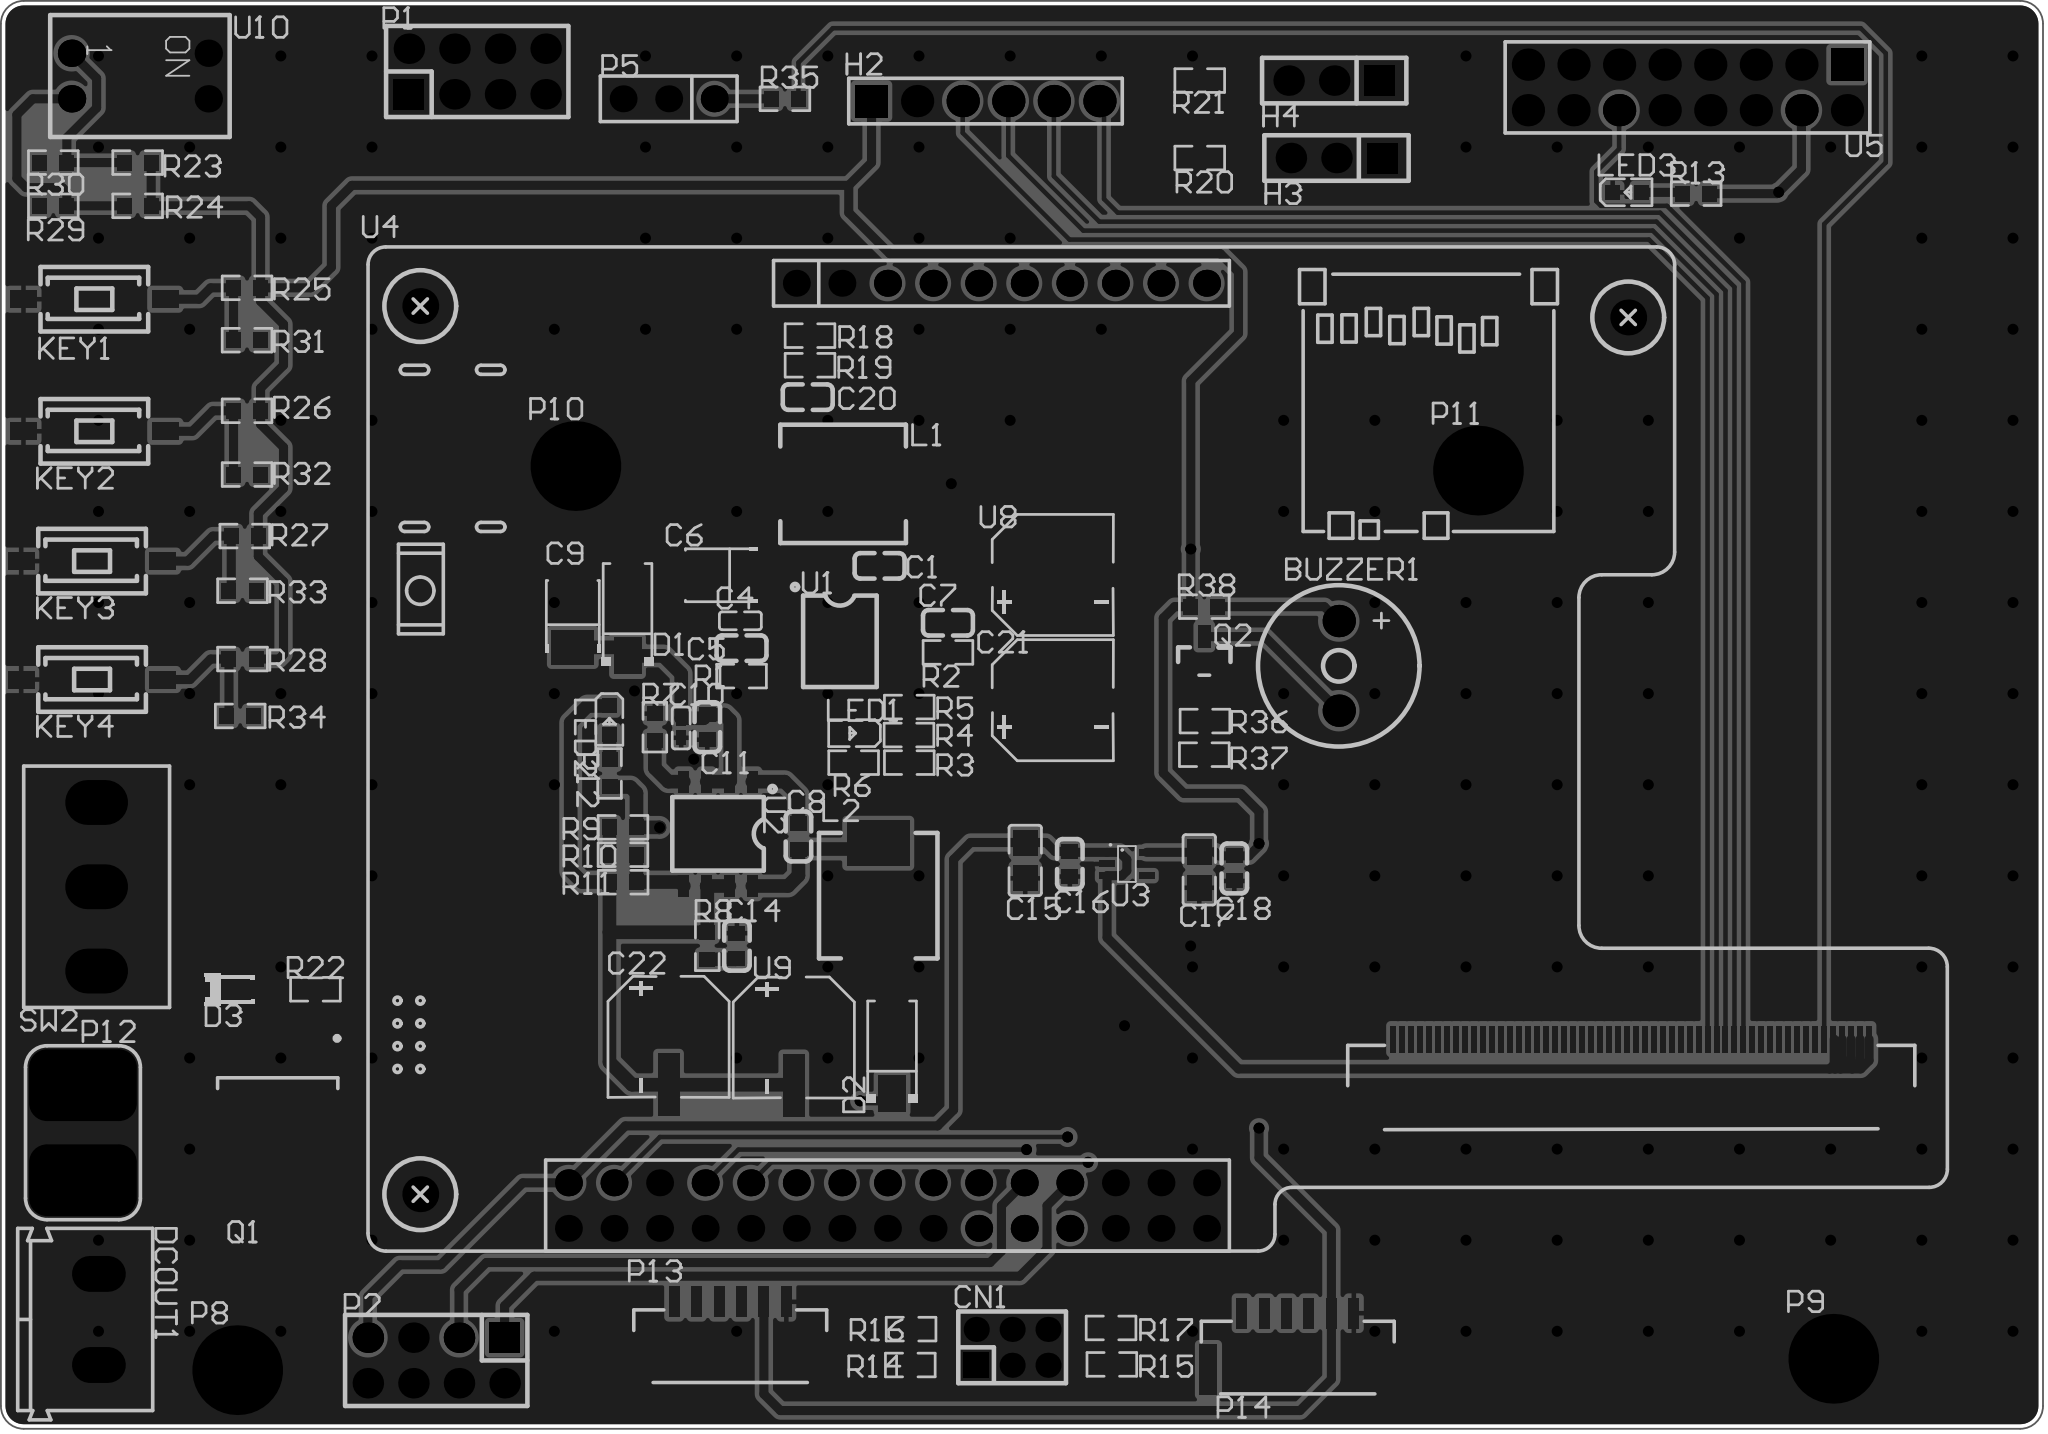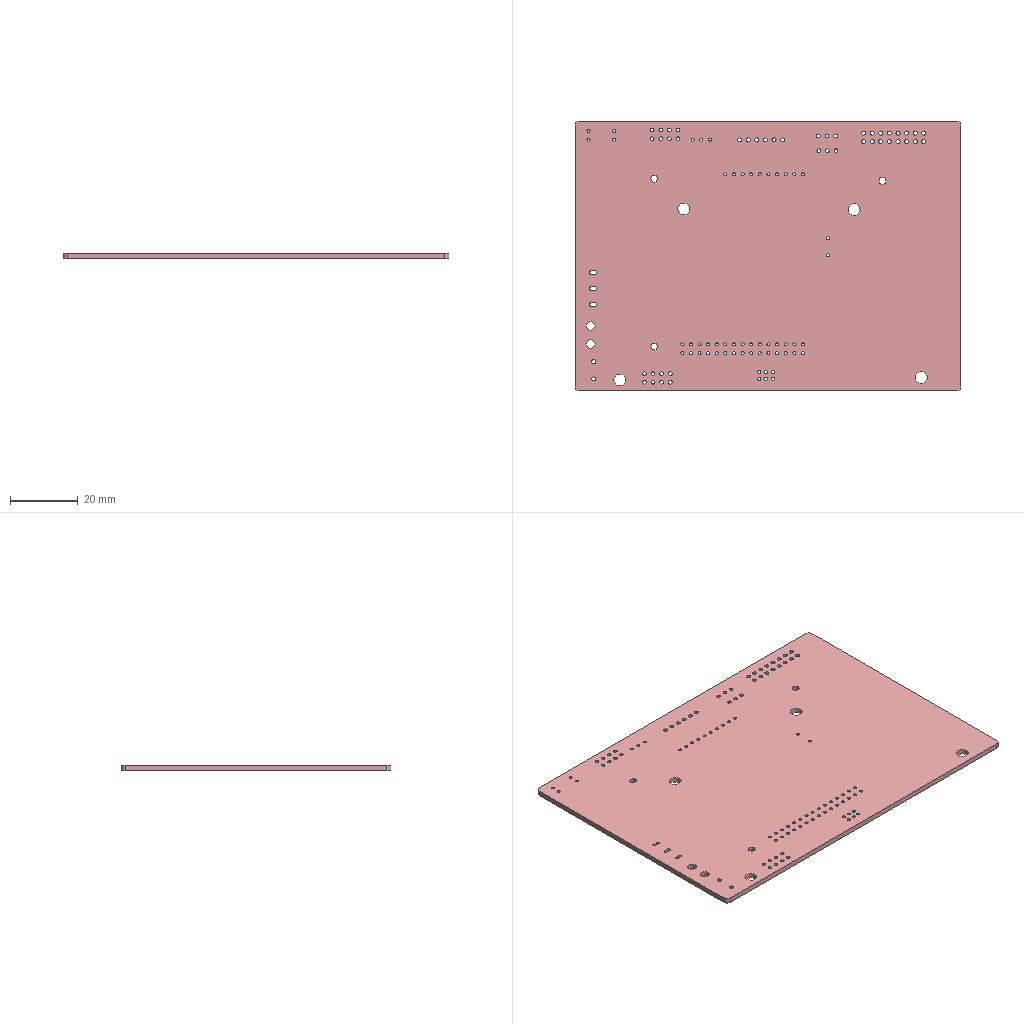Circuit board layout | Altium Designer | box 113.8 x 79.6 x 1.6 mm
Layer stack:
# Altium Designer layer stack of  (unit mm; dielectric type: 0 none, 1 core, 2 prepreg, 3 surface material)
index,name,kind,layer,copper_thickness_mm,dielectric_type,dielectric_thickness_mm,dielectric_material,dielectric_constant
0,Top Paste Mask Layer,other,,,,,,
1,Top Silkscreen Layer,other,,,,,,
2,Top Solder Mask Layer,dielectric,,,3,0.01,,3.3
3,Top Layer,copper,Top Layer,0.035,,,,
4,Dielectric1,dielectric,,,3,1.51,FR4,4.5
5,Bottom Layer,copper,Bottom Layer,0.035,,,,
6,Bottom Solder Mask Layer,dielectric,,,3,0.01,,3.3
7,Bottom Silkscreen Layer,other,,,,,,
8,Bottom Paste Mask Layer,other,,,,,,
# drill layer pairs: low layer,high layer
drill_pair,Top Layer,Bottom Layer
Part placement:
Designator,Comment,Layer,Footprint,Center-X(mm),Center-Y(mm),Rotation
BUZZER1,BEEP,TopLayer,BUZ-TH_BD9-P50-D0.6-FD,159.512,130.683,270
C1,100nF,TopLayer,C0603,133.925,136.26,0
C4,4.7uF,TopLayer,C0402,126.167,133.196,0
C5,100nF,TopLayer,C0603,126.232,131.672,0
C6,100uF,TopLayer,CAP-SMD_L3.5-W2.8-R-RD,124.934,135.736,0
C7,4.7nF,TopLayer,C0603,137.735,133.085,0
C8,100nF,TopLayer,C0603,129.405,121.169,270
C9,100uF,TopLayer,CAP-SMD_L3.5-W2.8-R-RD,116.832,133.615,270
C10,4.7uF,TopLayer,C0402,122.871,127.218,90
C11,100nF,TopLayer,C0603,124.325,127.265,90
C14,4.7nF,TopLayer,C0603,125.975,115.076,270
C15,10uF,TopLayer,C0805,142.04,119.833,90
C16,100nF,TopLayer,C0603,144.526,119.634,90
C17,10uF,TopLayer,C0805,151.738,119.309,90
C18,100nF,TopLayer,C0603,153.692,119.387,90
CN1,A2005WV-2x3P,TopLayer,HDR-TH_6P-P2.00-V-M-R2-C3-S2.00,141.311,92.679,0
D1,SS54,TopLayer,SMA_L4.4-W2.8-LS5.4-R-RD,119.879,133.742,90
D2,SS54,TopLayer,SMA_L4.4-W2.8-LS5.4-R-RD,134.62,109.347,90
D3,BZT52C16,TopLayer,SOD-123-L,97.79,112.649,180
DCOUT1,DCOUT1,TopLayer,KF/WJ/DG_301-2P-5.0MM,90.424,94.234,90
H2,2.54-1x6P straight pin,TopLayer,HDR-TH_6P-P2.54-V-M-1,139.827,162.179,0
H3,,TopLayer,HDR-TH_3P-P2.54-V-M,159.385,159.004,180
H4,,TopLayer,HDR-TH_3P-P2.54-V-M,159.258,163.322,180
KEY1,Tact switch 3x6x2.5mm,TopLayer,SW-SMD_L6.0-W3.6-LS8.0,90.17,151.13,180
KEY2,Tact switch 3x6x2.5mm,TopLayer,SW-SMD_L6.0-W3.6-LS8.0,90.17,143.764,180
KEY3,Tact switch 3x6x2.5mm,TopLayer,SW-SMD_L6.0-W3.6-LS8.0,90.043,136.525,180
KEY4,Tact switch 3x6x2.5mm,TopLayer,SW-SMD_L6.0-W3.6-LS8.0,90.043,129.921,180
LED1,LTST-C190KSKT,TopLayer,LED0603-RD,132.478,126.937,180
LED2,LTST-C190KSKT,TopLayer,LED0603-RD,118.864,127.646,270
LED3,LTST-C190KSKT,TopLayer,LED0603-RD,175.574,157.088,0
P1,Straight header 2X4P 2.54mm,TopLayer,HDR-TH_8P-P2.54-V-M-R2-C4-S2.54,111.506,163.83,0
P2,Straight header 2X4P 2.54mm,TopLayer,HDR-TH_8P-P2.54-V-M-R2-C4-S2.54,109.22,91.948,180
P5,Header-D-M 1x3P,TopLayer,HDR1X3-M,122.174,162.306,180
P8,,TopLayer,定位孔,98.13,91.406,0
P9,,TopLayer,定位孔,187.069,92.041,0
P10,,TopLayer,定位孔,116.976,141.825,0
P11,,TopLayer,定位孔,167.268,141.571,0
P12,XT60_Header,TopLayer,Wired_T-Header_ThroughHole,89.535,104.648,0
P13,GH1.25-6P,TopLayer,ECD-GH1.25-6P-SH,125.603,93.643,0
P14,GH1.25-6P,TopLayer,ECD-GH1.25-6P-SH,157.226,93.008,0
Q1,HY19P03,TopLayer,TO-252AA,100.387,106.635,270
Q2,S8050,TopLayer,SOT-23(SOT-23-3),152.019,131.064,0
SW2,SS-12D10L9,TopLayer,MTS-10x,90.297,118.364,90
U1,SCT2450CQSTER,TopLayer,ESOP-8_L4.9-W3.9-P1.27-LS6.0-BL-EP,131.713,132.053,270
U2,SCT2450CQSTER,TopLayer,ESOP-8_L4.9-W3.9-P1.27-LS6.0-BL-EP,124.924,121.316,180
U3,RT9013-33GU5,TopLayer,SC-70-5_L2.0-W1.3-P0.65-LS2.1-BR,147.701,119.634,180
U4,Loongson 2K0300 development board,TopLayer,龙芯2K0300久久派开发板,149.746,125.666,0
U5,2X8PIN2.54,TopLayer,HDR-TH_16P-P2.54-V-M-R2-C8-S2.54,178.943,162.941,180
R1,200kΩ,TopLayer,R0603,126.232,130.112,0
R2,20kΩ,TopLayer,R0603,137.735,131.434,0
R3,27kΩ,TopLayer,R0603,135.58,125.288,180
R4,27kΩ,TopLayer,R0603,135.563,126.826,0
R5,7.5kΩ,TopLayer,R0603,135.58,128.386,180
R6,10K,TopLayer,R0603,132.478,125.286,0
R7,200kΩ,TopLayer,R0603,121.403,127.265,270
R8,20kΩ,TopLayer,R0603,124.325,115.073,270
R9,51kΩ,TopLayer,R0603,119.626,121.677,0
R10,1.5kΩ,TopLayer,R0603,119.626,120.153,180
R11,7.5kΩ,TopLayer,R0603,119.634,118.618,0
R12,4.7kΩ,TopLayer,R0603,118.876,124.682,270
R13,2.7kΩ,TopLayer,R0603,179.427,157.017,180
R14,100Ω,TopLayer,R0603,135.636,91.694,0
R15,100Ω,TopLayer,R0603,146.867,91.728,180
R16,100Ω,TopLayer,R0603,135.679,93.695,180
R17,100Ω,TopLayer,R0603,146.823,93.76,0
R18,20kΩ,TopLayer,R0603,130.048,149.098,0
R19,200kΩ,TopLayer,R0603,130.048,147.447,180
R20,100Ω,TopLayer,R0603,151.765,159.004,180
R21,100Ω,TopLayer,R0603,151.765,163.322,180
R22,10K,TopLayer,R0603,102.489,112.649,180
R23,4.7kΩ,TopLayer,R0603,92.583,158.75,180
R24,4.7kΩ,TopLayer,R0603,92.583,156.337,180
R25,4.7kΩ,TopLayer,R0603,98.679,151.765,180
R26,4.7kΩ,TopLayer,R0603,98.679,144.907,180
R27,4.7kΩ,TopLayer,R0603,98.552,137.922,180
R28,4.7kΩ,TopLayer,R0603,98.425,131.064,180
R29,470Ω,TopLayer,R0603,87.884,156.337,180
R30,470Ω,TopLayer,R0603,87.884,158.75,180
R31,100Ω,TopLayer,R0603,98.679,148.844,0
R32,100Ω,TopLayer,R0603,98.679,141.351,0
R33,100Ω,TopLayer,R0603,98.425,134.874,0
R34,100Ω,TopLayer,R0603,98.298,127.889,0
R35,100Ω,TopLayer,R0603,128.651,162.306,180
R36,4.7kΩ,TopLayer,R0603,152.056,127.604,180
R37,1kΩ,TopLayer,R0603,152.019,125.73,180
R38,10Ω,TopLayer,R0603,152.019,133.985,0
C20,100nF,TopLayer,C0603,129.921,145.669,0
C21,47uF,TopLayer,CAP-SMD_BD6.3-L6.6-W6.6-LS7.3-FD,143.577,128.767,0
C22,47uF,TopLayer,CAP-SMD_BD6.3-L6.6-W6.6-LS7.3-FD,122.165,109.993,270
U8,220uF,TopLayer,CAP-SMD_BD6.3-L6.6-W6.6-LS7.2-FD,143.577,135.752,0
U9,220uF,TopLayer,CAP-SMD_BD6.3-L6.6-W6.6-LS7.2-FD,129.144,109.955,270
L1,4.7uH,TopLayer,IND-SMD_L7.0-W6.6_VCMT063T,131.893,140.832,0
L2,4.7uH,TopLayer,IND-SMD_L7.0-W6.6_VCMT063T,133.85,117.867,270
U10,2-position DIP switch,TopLayer,SW-TH_4P-L9.9-W6.8-P7.62-BL,92.71,163.576,270
Pad and via stacks:
# Altium Designer via and pad stacks of  (unit mm). Each distinct definition once, with the count of objects using it.
# via: kind,start_layer,end_layer,hole_mm,diameter_mm,mode(0 simple;1 top-mid-bottom;2 full stack),diameter_per_layer,count,example_net
# pad: kind,layer,hole_mm,hole_type(0 round;1 square;2 slot),plating,top_size,top_shape(1 round;2 rect;3 octagon;9 rounded rect),mid_size,bottom_size,mode,footprint,size_per_layer,count,example
pad,Multi-Layer,1,0,plated,1.8x1.8,1,1.8x1.8,1.8x1.8,0,BUZ-TH_BD9-P50-D0.6-FD,,2,BUZZER1.2
pad,Multi-Layer,0.9,0,plated,1.4x1.4,1,1.4x1.4,1.4x1.4,0,HDR-TH_6P-P2.00-V-M-R2-C3-S2.00,,5,CN1.6
pad,Multi-Layer,0.9,0,plated,1.4x1.4,2,1.4x1.4,1.4x1.4,0,HDR-TH_6P-P2.00-V-M-R2-C3-S2.00,,1,CN1.1
pad,Multi-Layer,1.2,0,plated,2x3,1,2x3,2x3,0,KF/WJ/DG 301-2P-5.0MM,,2,DCOUT1.1
pad,Multi-Layer,1.2,0,plated,1.8x1.8,1,1.8x1.8,1.8x1.8,0,HDR-TH_6P-P2.54-V-M-1,,5,H2.6
pad,Multi-Layer,1.2,0,plated,1.8x1.8,2,1.8x1.8,1.8x1.8,0,HDR-TH_6P-P2.54-V-M-1,,1,H2.1
pad,Multi-Layer,1.1,0,plated,1.7x1.7,2,1.7x1.7,1.7x1.7,0,HDR-TH_3P-P2.54-V-M,,2,H3.1
pad,Multi-Layer,1.1,0,plated,1.7x1.7,1,1.7x1.7,1.7x1.7,0,HDR-TH_3P-P2.54-V-M,,4,H3.2
pad,Multi-Layer,1.1,0,plated,1.7x1.7,2,1.7x1.7,1.7x1.7,0,HDR-TH_8P-P2.54-V-M-R2-C4-S2.54,,2,P1.1
pad,Multi-Layer,1.1,0,plated,1.7x1.7,1,1.7x1.7,1.7x1.7,0,HDR-TH_8P-P2.54-V-M-R2-C4-S2.54,,14,P1.2
pad,Multi-Layer,0.9,0,plated,1.5x1.5,1,1.5x1.5,1.5x1.5,0,HDR1X3-M,,3,P5.1
pad,Multi-Layer,3.5,0,plated,5x5,1,5x5,5x5,0,\u00B6\u00A8\u00CE\u00BB\u00BF\u00D7,,4,P8.1
pad,Multi-Layer,2.6,0,plated,6x4,9,6x4,6x4,0,Wired T-Header ThroughHole,,2,P12.1
pad,Multi-Layer,1,2,unplated,3.5x2.5,1,3.5x2.5,3.5x2.5,0,MTS-10x,,3,SW2.3
pad,Multi-Layer,0.9,0,plated,1.5x1.5,1,1.5x1.5,1.5x1.5,0,\u00C1\u00FA\u00D0\u00BE2K0300\u00BE\u00C3\u00BE\u00C3\u00C5\u00C9\u00BF\u00AA\u00B7\u00A2\u00B0\u00E5,,40,U4.31
pad,Multi-Layer,2,0,unplated,2x2,1,2x2,2x2,0,\u00C1\u00FA\u00D0\u00BE2K0300\u00BE\u00C3\u00BE\u00C3\u00C5\u00C9\u00BF\u00AA\u00B7\u00A2\u00B0\u00E5,,3,U4.0
pad,Multi-Layer,1.2,0,plated,1.8x1.8,1,1.8x1.8,1.8x1.8,0,HDR-TH_16P-P2.54-V-M-R2-C8-S2.54,,15,U5.16
pad,Multi-Layer,1.2,0,plated,1.8x1.8,2,1.8x1.8,1.8x1.8,0,HDR-TH_16P-P2.54-V-M-R2-C8-S2.54,,1,U5.1
pad,Multi-Layer,0.9144,0,plated,1.524x1.524,1,1.524x1.524,1.524x1.524,0,SW-TH_4P-L9.9-W6.8-P7.62-BL,,4,U10.1
pad,Top Layer,0,0,plated,0.8x0.9,2,0.8x0.9,0.8x0.9,0,C0603,,18,C1.2
pad,Top Layer,0,0,plated,0.7901x0.54,2,0.7901x0.54,0.7901x0.54,0,C0402,,4,C4.2
pad,Top Layer,0,0,plated,1.9x2.376,2,1.9x2.376,1.9x2.376,0,CAP-SMD_L3.5-W2.8-R-RD,,4,C6.1
pad,Top Layer,0,0,plated,1.41x1.35,2,1.41x1.35,1.41x1.35,0,C0805,,4,C15.2
pad,Top Layer,0,0,plated,2.062x1.539,2,2.062x1.539,2.062x1.539,0,SMA_L4.4-W2.8-LS5.4-R-RD,,4,D1.1
pad,Top Layer,0,0,unplated,1x0.85,2,1x0.85,1x0.85,0,SOD-123-L,,2,D3.K
pad,Top Layer,0,0,plated,1.5x1,2,1.5x1,1.5x1,0,SW-SMD_L6.0-W3.6-LS8.0,,8,KEY1.1
pad,Top Layer,0,0,plated,0.8x0.8,2,0.8x0.8,0.8x0.8,0,LED0603-RD,,6,LED1.2
pad,Top Layer,0,0,plated,0.6x1.7,2,0.6x1.7,0.6x1.7,0,ECD-GH1.25-6P-SH,,12,P13.6
pad,Top Layer,0,0,plated,1x2.8,2,1x2.8,1x2.8,0,ECD-GH1.25-6P-SH,,4,P13.0
pad,Top Layer,0,0,plated,0.95x2.2,2,0.95x2.2,0.95x2.2,0,TO-252AA,,2,Q1.3
pad,Top Layer,0,0,plated,5.5x6.7,2,5.5x6.7,5.5x6.7,0,TO-252AA,,1,Q1.1
pad,Top Layer,0,0,plated,0.7x1.25,2,0.7x1.25,0.7x1.25,0,SOT-23(SOT-23-3),,3,Q2.3
pad,Top Layer,0,0,plated,0.6x1.2,2,0.6x1.2,0.6x1.2,0,ESOP-8_L4.9-W3.9-P1.27-LS6.0-BL-EP,,16,U1.1
pad,Top Layer,0,0,plated,3.3x2.4,2,3.3x2.4,3.3x2.4,0,ESOP-8_L4.9-W3.9-P1.27-LS6.0-BL-EP,,2,U1.9
pad,Top Layer,0,0,plated,0.35x0.85,2,0.35x0.85,0.35x0.85,0,SC-70-5_L2.0-W1.3-P0.65-LS2.1-BR,,5,U3.1
pad,Top Layer,0,0,plated,2.5x2.5,2,2.5x2.5,2.5x2.5,0,\u00C1\u00FA\u00D0\u00BE2K0300\u00BE\u00C3\u00BE\u00C3\u00C5\u00C9\u00BF\u00AA\u00B7\u00A2\u00B0\u00E5,,2,U4.41
pad,Top Layer,0,0,plated,0.3048x1.5,2,0.3048x1.5,0.3048x1.5,0,\u00C1\u00FA\u00D0\u00BE2K0300\u00BE\u00C3\u00BE\u00C3\u00C5\u00C9\u00BF\u00AA\u00B7\u00A2\u00B0\u00E5,,54,U4.72
pad,Top Layer,0,0,plated,0.8065x0.864,2,0.8065x0.864,0.8065x0.864,0,R0603,,76,R1.2
pad,Top Layer,0,0,plated,3.5x1.2,2,3.5x1.2,3.5x1.2,0,CAP-SMD_BD6.3-L6.6-W6.6-LS7.3-FD,,4,C21.2
pad,Top Layer,0,0,plated,3.5x1.2,2,3.5x1.2,3.5x1.2,0,CAP-SMD_BD6.3-L6.6-W6.6-LS7.2-FD,,4,U8.2
pad,Top Layer,0,0,plated,2.55x3.5,2,2.55x3.5,2.55x3.5,0,IND-SMD_L7.0-W6.6_VCMT063T,,4,L1.1
via,Top Layer,Bottom Layer,0.3048,0.61,0,,194,$1N2679
Copper pours:
name,layer,net,type(0 solid;1 hatched;2 none)
Top Layer-GND,Top Layer,GND,0
Bottom Layer-GND,Bottom Layer,GND,0